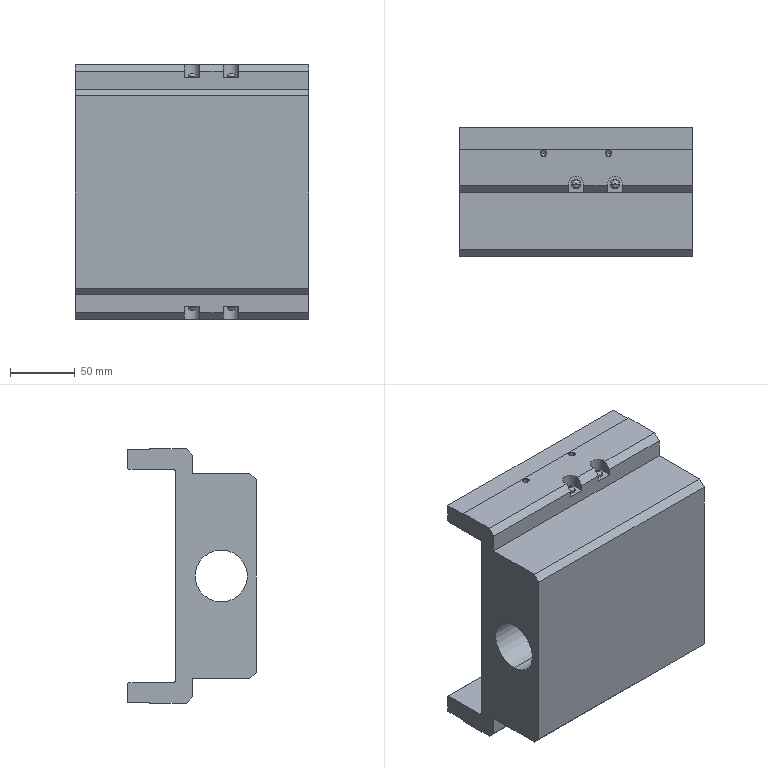Part | STEP file | ISPB-WXM-WA-750-10-650-T4-N-AQ-EB-G3-^-Part-2 | 1 solid | 178 faces | box 180 x 99 x 196 mm | volume 1807834 mm3 | cylinder 68 | plane 54 | cone 48 | other 8 | commonest cylinder face diameters 6.647 x16 8 x12 4.134 x8 6 x8 6.9 x8 7.5 x8